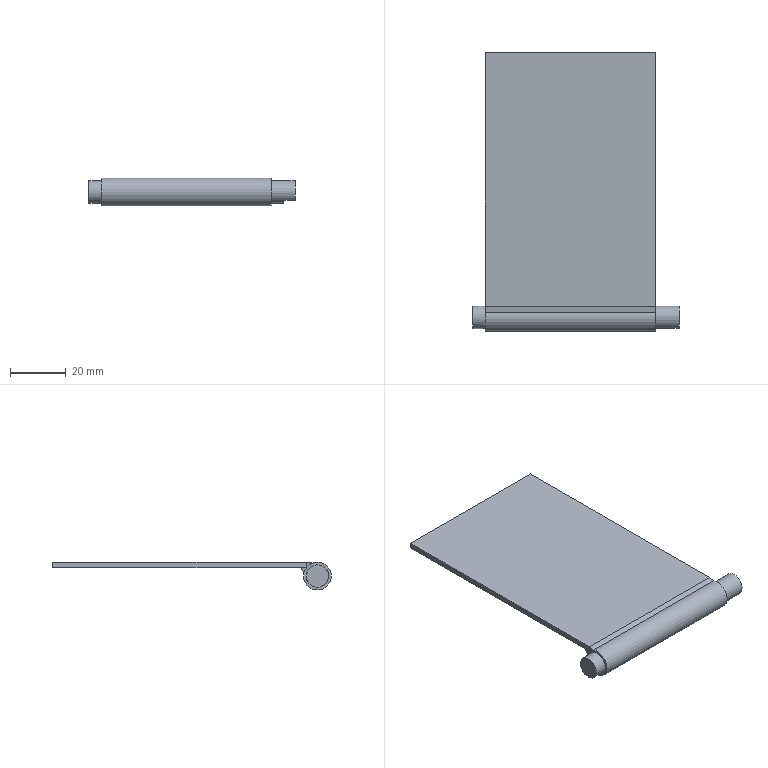Part | NX | features EXTRUDE 4, DATUM_CSYS 2, FSET 2, FILLET_WELD 1, HOLE PACKAGE 1, SIMPLE HOLE 1, SKETCH 1, SYMBOLIC_THREAD 1, WELD_GROOVE 1 | 4 solids | 28 faces | box 74 x 100 x 10 mm | volume 16601 mm3 | plane 19 | cylinder 6 | cone 2 | spline 1 | commonest cylinder face diameters 10 x3 8 x2 4.2 x1
STEP:
#1=CARTESIAN_POINT('',(-30.5,1.769,4.677));
#2=VERTEX_POINT('',#1);
#3=CARTESIAN_POINT('',(30.5,1.769,4.677));
#4=VERTEX_POINT('',#3);
#5=CARTESIAN_POINT('',(-0.000000001,1.769,4.677));
#6=DIRECTION('',(-1.,0.,0.));
#7=VECTOR('',#6,1000.);
#8=LINE('',#5,#7);
#9=EDGE_CURVE('',#2,#4,#8,.F.);
#10=ORIENTED_EDGE('',*,*,#9,.F.);
#11=CARTESIAN_POINT('',(-30.5,4.,3.));
#12=VERTEX_POINT('',#11);
#13=CARTESIAN_POINT('',(-30.5,0.,0.));
#14=DIRECTION('',(1.,0.,0.));
#15=DIRECTION('',(0.,1.,0.));
#16=AXIS2_PLACEMENT_3D('',#13,#14,#15);
#17=CIRCLE('',#16,5.);
#18=EDGE_CURVE('',#12,#2,#17,.T.);
#19=ORIENTED_EDGE('',*,*,#18,.F.);
#20=CARTESIAN_POINT('',(30.5,4.,3.));
#21=VERTEX_POINT('',#20);
#22=CARTESIAN_POINT('',(30.5,4.,3.));
#23=DIRECTION('',(-1.,0.,0.));
#24=VECTOR('',#23,1000.);
#25=LINE('',#22,#24);
#26=EDGE_CURVE('',#12,#21,#25,.F.);
#27=ORIENTED_EDGE('',*,*,#26,.T.);
#28=CARTESIAN_POINT('',(30.5,0.,0.));
#29=DIRECTION('',(1.,0.,0.));
#30=DIRECTION('',(0.,1.,0.));
#31=AXIS2_PLACEMENT_3D('',#28,#29,#30);
#32=CIRCLE('',#31,5.);
#33=EDGE_CURVE('',#21,#4,#32,.T.);
#34=ORIENTED_EDGE('',*,*,#33,.T.);
#35=EDGE_LOOP('',(#10,#19,#27,#34));
#36=FACE_BOUND('',#35,.T.);
#37=CARTESIAN_POINT('',(30.5,0.,0.));
#38=DIRECTION('',(-1.,0.,0.));
#39=DIRECTION('',(0.,0.,1.));
#40=AXIS2_PLACEMENT_3D('',#37,#38,#39);
#41=CYLINDRICAL_SURFACE('',#40,5.);
#42=ADVANCED_FACE('',(#36),#41,.F.);
#43=CARTESIAN_POINT('',(-30.5,4.,5.));
#44=VERTEX_POINT('',#43);
#45=CARTESIAN_POINT('',(-30.5,4.,3.));
#46=DIRECTION('',(0.,0.,1.));
#47=VECTOR('',#46,1000.);
#48=LINE('',#45,#47);
#49=EDGE_CURVE('',#12,#44,#48,.T.);
#50=ORIENTED_EDGE('',*,*,#49,.T.);
#51=CARTESIAN_POINT('',(30.5,4.,5.));
#52=VERTEX_POINT('',#51);
#53=CARTESIAN_POINT('',(-30.5,4.,5.));
#54=DIRECTION('',(1.,0.,0.));
#55=VECTOR('',#54,1000.);
#56=LINE('',#53,#55);
#57=EDGE_CURVE('',#44,#52,#56,.T.);
#58=ORIENTED_EDGE('',*,*,#57,.T.);
#59=CARTESIAN_POINT('',(30.5,4.,3.));
#60=DIRECTION('',(0.,0.,1.));
#61=VECTOR('',#60,1000.);
#62=LINE('',#59,#61);
#63=EDGE_CURVE('',#21,#52,#62,.T.);
#64=ORIENTED_EDGE('',*,*,#63,.F.);
#65=ORIENTED_EDGE('',*,*,#26,.F.);
#66=EDGE_LOOP('',(#50,#58,#64,#65));
#67=FACE_BOUND('',#66,.T.);
#68=CARTESIAN_POINT('',(-30.5,4.,3.));
#69=DIRECTION('',(0.,-1.,0.));
#70=DIRECTION('',(1.,0.,0.));
#71=AXIS2_PLACEMENT_3D('',#68,#69,#70);
#72=PLANE('',#71);
#73=ADVANCED_FACE('',(#67),#72,.F.);
#74=ORIENTED_EDGE('',*,*,#9,.T.);
#75=CARTESIAN_POINT('',(30.5,1.769,4.677));
#76=CARTESIAN_POINT('',(30.5,2.513,4.784));
#77=CARTESIAN_POINT('',(30.5,3.256,4.892));
#78=CARTESIAN_POINT('',(30.5,4.,5.));
#79=B_SPLINE_CURVE_WITH_KNOTS('',3,(#75,#76,#77,#78),.UNSPECIFIED.,.F.,.F.,(4,4),(0.,0.002254),.UNSPECIFIED.);
#80=EDGE_CURVE('',#4,#52,#79,.T.);
#81=ORIENTED_EDGE('',*,*,#80,.T.);
#82=ORIENTED_EDGE('',*,*,#57,.F.);
#83=CARTESIAN_POINT('',(-30.5,4.,5.));
#84=CARTESIAN_POINT('',(-30.5,3.256,4.892));
#85=CARTESIAN_POINT('',(-30.5,2.513,4.784));
#86=CARTESIAN_POINT('',(-30.5,1.769,4.677));
#87=B_SPLINE_CURVE_WITH_KNOTS('',3,(#83,#84,#85,#86),.UNSPECIFIED.,.F.,.F.,(4,4),(0.,0.002254),.UNSPECIFIED.);
#88=EDGE_CURVE('',#44,#2,#87,.T.);
#89=ORIENTED_EDGE('',*,*,#88,.T.);
#90=EDGE_LOOP('',(#74,#81,#82,#89));
#91=FACE_BOUND('',#90,.T.);
#92=CARTESIAN_POINT('',(-30.75,4.112,5.016));
#93=CARTESIAN_POINT('',(-30.75,3.293,4.898));
#94=CARTESIAN_POINT('',(-30.75,2.475,4.779));
#95=CARTESIAN_POINT('',(-30.75,1.657,4.66));
#96=CARTESIAN_POINT('',(-28.188,4.112,5.016));
#97=CARTESIAN_POINT('',(-28.187,3.293,4.898));
#98=CARTESIAN_POINT('',(-28.188,2.475,4.779));
#99=CARTESIAN_POINT('',(-28.187,1.657,4.66));
#100=CARTESIAN_POINT('',(-23.062,4.112,5.016));
#101=CARTESIAN_POINT('',(-23.063,3.293,4.898));
#102=CARTESIAN_POINT('',(-23.062,2.475,4.779));
#103=CARTESIAN_POINT('',(-23.062,1.657,4.66));
#104=CARTESIAN_POINT('',(-12.812,4.112,5.016));
#105=CARTESIAN_POINT('',(-12.813,3.293,4.898));
#106=CARTESIAN_POINT('',(-12.812,2.475,4.779));
#107=CARTESIAN_POINT('',(-12.813,1.657,4.66));
#108=CARTESIAN_POINT('',(-2.562,4.112,5.016));
#109=CARTESIAN_POINT('',(-2.563,3.293,4.898));
#110=CARTESIAN_POINT('',(-2.562,2.475,4.779));
#111=CARTESIAN_POINT('',(-2.563,1.657,4.66));
#112=CARTESIAN_POINT('',(7.687,4.112,5.016));
#113=CARTESIAN_POINT('',(7.688,3.293,4.898));
#114=CARTESIAN_POINT('',(7.687,2.475,4.779));
#115=CARTESIAN_POINT('',(7.687,1.657,4.66));
#116=CARTESIAN_POINT('',(15.375,4.112,5.016));
#117=CARTESIAN_POINT('',(15.375,3.293,4.898));
#118=CARTESIAN_POINT('',(15.375,2.475,4.779));
#119=CARTESIAN_POINT('',(15.375,1.657,4.66));
#120=CARTESIAN_POINT('',(23.062,4.112,5.016));
#121=CARTESIAN_POINT('',(23.063,3.293,4.898));
#122=CARTESIAN_POINT('',(23.062,2.475,4.779));
#123=CARTESIAN_POINT('',(23.062,1.657,4.66));
#124=CARTESIAN_POINT('',(28.188,4.112,5.016));
#125=CARTESIAN_POINT('',(28.187,3.293,4.898));
#126=CARTESIAN_POINT('',(28.188,2.475,4.779));
#127=CARTESIAN_POINT('',(28.187,1.657,4.66));
#128=CARTESIAN_POINT('',(30.75,4.112,5.016));
#129=CARTESIAN_POINT('',(30.75,3.293,4.898));
#130=CARTESIAN_POINT('',(30.75,2.475,4.779));
#131=CARTESIAN_POINT('',(30.75,1.657,4.66));
#132=B_SPLINE_SURFACE_WITH_KNOTS('',3,3,((#92,#93,#94,#95),(#96,#97,#98,#99),(#100,#101,#102,#103),(#104,#105,#106,#107),(#108,#109,#110,#111),(#112,#113,#114,#115),(#116,#117,#118,#119),(#120,#121,#122,#123),(#124,#125,#126,#127),(#128,#129,#130,#131)),.UNSPECIFIED.,.F.,.F.,.F.,(4,1,1,1,1,1,1,4),(4,4),(0.,0.125,0.25,0.5,0.625,0.75,0.875,1.),(0.,1.),.UNSPECIFIED.);
#133=ADVANCED_FACE('',(#91),#132,.F.);
#134=ORIENTED_EDGE('',*,*,#18,.T.);
#135=ORIENTED_EDGE('',*,*,#88,.F.);
#136=ORIENTED_EDGE('',*,*,#49,.F.);
#137=EDGE_LOOP('',(#134,#135,#136));
#138=FACE_BOUND('',#137,.T.);
#139=CARTESIAN_POINT('',(-30.5,4.,3.));
#140=DIRECTION('',(1.,0.,0.));
#141=DIRECTION('',(0.,0.,-1.));
#142=AXIS2_PLACEMENT_3D('',#139,#140,#141);
#143=PLANE('',#142);
#144=ADVANCED_FACE('',(#138),#143,.F.);
#145=ORIENTED_EDGE('',*,*,#33,.F.);
#146=ORIENTED_EDGE('',*,*,#63,.T.);
#147=ORIENTED_EDGE('',*,*,#80,.F.);
#148=EDGE_LOOP('',(#145,#146,#147));
#149=FACE_BOUND('',#148,.T.);
#150=CARTESIAN_POINT('',(30.5,4.,3.));
#151=DIRECTION('',(-1.,0.,0.));
#152=DIRECTION('',(0.,0.,1.));
#153=AXIS2_PLACEMENT_3D('',#150,#151,#152);
#154=PLANE('',#153);
#155=ADVANCED_FACE('',(#149),#154,.F.);
#156=CLOSED_SHELL('',(#42,#73,#133,#144,#155));
#157=MANIFOLD_SOLID_BREP('',#156);
#158=CARTESIAN_POINT('',(-30.5,95.,3.));
#159=VERTEX_POINT('',#158);
#160=CARTESIAN_POINT('',(-30.5,95.,5.));
#161=VERTEX_POINT('',#160);
#162=CARTESIAN_POINT('',(-30.5,95.,3.));
#163=DIRECTION('',(0.,0.,1.));
#164=VECTOR('',#163,1000.);
#165=LINE('',#162,#164);
#166=EDGE_CURVE('',#159,#161,#165,.T.);
#167=ORIENTED_EDGE('',*,*,#166,.F.);
#168=CARTESIAN_POINT('',(-30.5,4.,3.));
#169=VERTEX_POINT('',#168);
#170=CARTESIAN_POINT('',(-30.5,95.,3.));
#171=DIRECTION('',(0.,-1.,0.));
#172=VECTOR('',#171,1000.);
#173=LINE('',#170,#172);
#174=EDGE_CURVE('',#159,#169,#173,.T.);
#175=ORIENTED_EDGE('',*,*,#174,.T.);
#176=CARTESIAN_POINT('',(-30.5,4.,5.));
#177=VERTEX_POINT('',#176);
#178=CARTESIAN_POINT('',(-30.5,4.,3.));
#179=DIRECTION('',(0.,0.,1.));
#180=VECTOR('',#179,1000.);
#181=LINE('',#178,#180);
#182=EDGE_CURVE('',#169,#177,#181,.T.);
#183=ORIENTED_EDGE('',*,*,#182,.T.);
#184=CARTESIAN_POINT('',(-30.5,95.,5.));
#185=DIRECTION('',(0.,1.,0.));
#186=VECTOR('',#185,1000.);
#187=LINE('',#184,#186);
#188=EDGE_CURVE('',#161,#177,#187,.F.);
#189=ORIENTED_EDGE('',*,*,#188,.F.);
#190=EDGE_LOOP('',(#167,#175,#183,#189));
#191=FACE_BOUND('',#190,.T.);
#192=CARTESIAN_POINT('',(-30.5,95.,3.));
#193=DIRECTION('',(-1.,0.,0.));
#194=DIRECTION('',(0.,-1.,0.));
#195=AXIS2_PLACEMENT_3D('',#192,#193,#194);
#196=PLANE('',#195);
#197=ADVANCED_FACE('',(#191),#196,.T.);
#198=ORIENTED_EDGE('',*,*,#182,.F.);
#199=CARTESIAN_POINT('',(30.5,4.,3.));
#200=VERTEX_POINT('',#199);
#201=CARTESIAN_POINT('',(-30.5,4.,3.));
#202=DIRECTION('',(1.,0.,0.));
#203=VECTOR('',#202,1000.);
#204=LINE('',#201,#203);
#205=EDGE_CURVE('',#169,#200,#204,.T.);
#206=ORIENTED_EDGE('',*,*,#205,.T.);
#207=CARTESIAN_POINT('',(30.5,4.,5.));
#208=VERTEX_POINT('',#207);
#209=CARTESIAN_POINT('',(30.5,4.,3.));
#210=DIRECTION('',(0.,0.,1.));
#211=VECTOR('',#210,1000.);
#212=LINE('',#209,#211);
#213=EDGE_CURVE('',#200,#208,#212,.T.);
#214=ORIENTED_EDGE('',*,*,#213,.T.);
#215=CARTESIAN_POINT('',(-30.5,4.,5.));
#216=DIRECTION('',(1.,0.,0.));
#217=VECTOR('',#216,1000.);
#218=LINE('',#215,#217);
#219=EDGE_CURVE('',#177,#208,#218,.T.);
#220=ORIENTED_EDGE('',*,*,#219,.F.);
#221=EDGE_LOOP('',(#198,#206,#214,#220));
#222=FACE_BOUND('',#221,.T.);
#223=CARTESIAN_POINT('',(-30.5,4.,3.));
#224=DIRECTION('',(0.,-1.,0.));
#225=DIRECTION('',(1.,0.,0.));
#226=AXIS2_PLACEMENT_3D('',#223,#224,#225);
#227=PLANE('',#226);
#228=ADVANCED_FACE('',(#222),#227,.T.);
#229=ORIENTED_EDGE('',*,*,#213,.F.);
#230=CARTESIAN_POINT('',(30.5,95.,3.));
#231=VERTEX_POINT('',#230);
#232=CARTESIAN_POINT('',(30.5,95.,3.));
#233=DIRECTION('',(0.,-1.,0.));
#234=VECTOR('',#233,1000.);
#235=LINE('',#232,#234);
#236=EDGE_CURVE('',#231,#200,#235,.T.);
#237=ORIENTED_EDGE('',*,*,#236,.F.);
#238=CARTESIAN_POINT('',(30.5,95.,5.));
#239=VERTEX_POINT('',#238);
#240=CARTESIAN_POINT('',(30.5,95.,3.));
#241=DIRECTION('',(0.,0.,1.));
#242=VECTOR('',#241,1000.);
#243=LINE('',#240,#242);
#244=EDGE_CURVE('',#231,#239,#243,.T.);
#245=ORIENTED_EDGE('',*,*,#244,.T.);
#246=CARTESIAN_POINT('',(30.5,95.,5.));
#247=DIRECTION('',(0.,1.,0.));
#248=VECTOR('',#247,1000.);
#249=LINE('',#246,#248);
#250=EDGE_CURVE('',#239,#208,#249,.F.);
#251=ORIENTED_EDGE('',*,*,#250,.T.);
#252=EDGE_LOOP('',(#229,#237,#245,#251));
#253=FACE_BOUND('',#252,.T.);
#254=CARTESIAN_POINT('',(30.5,95.,3.));
#255=DIRECTION('',(-1.,0.,0.));
#256=DIRECTION('',(0.,-1.,0.));
#257=AXIS2_PLACEMENT_3D('',#254,#255,#256);
#258=PLANE('',#257);
#259=ADVANCED_FACE('',(#253),#258,.F.);
#260=CARTESIAN_POINT('',(-30.5,95.,3.));
#261=DIRECTION('',(1.,0.,0.));
#262=VECTOR('',#261,1000.);
#263=LINE('',#260,#262);
#264=EDGE_CURVE('',#159,#231,#263,.T.);
#265=ORIENTED_EDGE('',*,*,#264,.F.);
#266=ORIENTED_EDGE('',*,*,#166,.T.);
#267=CARTESIAN_POINT('',(-30.5,95.,5.));
#268=DIRECTION('',(1.,0.,0.));
#269=VECTOR('',#268,1000.);
#270=LINE('',#267,#269);
#271=EDGE_CURVE('',#161,#239,#270,.T.);
#272=ORIENTED_EDGE('',*,*,#271,.T.);
#273=ORIENTED_EDGE('',*,*,#244,.F.);
#274=EDGE_LOOP('',(#265,#266,#272,#273));
#275=FACE_BOUND('',#274,.T.);
#276=CARTESIAN_POINT('',(-30.5,95.,3.));
#277=DIRECTION('',(0.,-1.,0.));
#278=DIRECTION('',(1.,0.,0.));
#279=AXIS2_PLACEMENT_3D('',#276,#277,#278);
#280=PLANE('',#279);
#281=ADVANCED_FACE('',(#275),#280,.F.);
#282=ORIENTED_EDGE('',*,*,#250,.F.);
#283=ORIENTED_EDGE('',*,*,#271,.F.);
#284=ORIENTED_EDGE('',*,*,#188,.T.);
#285=ORIENTED_EDGE('',*,*,#219,.T.);
#286=EDGE_LOOP('',(#282,#283,#284,#285));
#287=FACE_BOUND('',#286,.T.);
#288=CARTESIAN_POINT('',(-30.5,95.,5.));
#289=DIRECTION('',(0.,0.,1.));
#290=DIRECTION('',(1.,0.,0.));
#291=AXIS2_PLACEMENT_3D('',#288,#289,#290);
#292=PLANE('',#291);
#293=ADVANCED_FACE('',(#287),#292,.T.);
#294=ORIENTED_EDGE('',*,*,#236,.T.);
#295=ORIENTED_EDGE('',*,*,#205,.F.);
#296=ORIENTED_EDGE('',*,*,#174,.F.);
#297=ORIENTED_EDGE('',*,*,#264,.T.);
#298=EDGE_LOOP('',(#294,#295,#296,#297));
#299=FACE_BOUND('',#298,.T.);
#300=CARTESIAN_POINT('',(-30.5,95.,3.));
#301=DIRECTION('',(0.,0.,1.));
#302=DIRECTION('',(1.,0.,0.));
#303=AXIS2_PLACEMENT_3D('',#300,#301,#302);
#304=PLANE('',#303);
#305=ADVANCED_FACE('',(#299),#304,.F.);
#306=CLOSED_SHELL('',(#197,#228,#259,#281,#293,#305));
#307=MANIFOLD_SOLID_BREP('',#306);
#308=CARTESIAN_POINT('',(-30.5,6.,3.));
#309=VERTEX_POINT('',#308);
#310=CARTESIAN_POINT('',(-30.5,4.,3.));
#311=VERTEX_POINT('',#310);
#312=CARTESIAN_POINT('',(-30.5,95.,3.));
#313=DIRECTION('',(0.,-1.,0.));
#314=VECTOR('',#313,1000.);
#315=LINE('',#312,#314);
#316=EDGE_CURVE('',#309,#311,#315,.T.);
#317=ORIENTED_EDGE('',*,*,#316,.F.);
#318=CARTESIAN_POINT('',(-30.5,4.852,1.206));
#319=VERTEX_POINT('',#318);
#320=CARTESIAN_POINT('',(-30.5,5.426,2.103));
#321=DIRECTION('',(0.,-0.5387,-0.8425));
#322=VECTOR('',#321,1000.);
#323=LINE('',#320,#322);
#324=EDGE_CURVE('',#309,#319,#323,.T.);
#325=ORIENTED_EDGE('',*,*,#324,.T.);
#326=CARTESIAN_POINT('',(-30.5,0.,0.));
#327=DIRECTION('',(1.,0.,0.));
#328=DIRECTION('',(0.,1.,0.));
#329=AXIS2_PLACEMENT_3D('',#326,#327,#328);
#330=CIRCLE('',#329,5.);
#331=EDGE_CURVE('',#319,#311,#330,.T.);
#332=ORIENTED_EDGE('',*,*,#331,.T.);
#333=EDGE_LOOP('',(#317,#325,#332));
#334=FACE_BOUND('',#333,.T.);
#335=CARTESIAN_POINT('',(-30.5,4.,3.));
#336=DIRECTION('',(1.,0.,0.));
#337=DIRECTION('',(0.,1.,0.));
#338=AXIS2_PLACEMENT_3D('',#335,#336,#337);
#339=PLANE('',#338);
#340=ADVANCED_FACE('',(#334),#339,.F.);
#341=CARTESIAN_POINT('',(30.5,6.,3.));
#342=VERTEX_POINT('',#341);
#343=CARTESIAN_POINT('',(30.5,4.,3.));
#344=VERTEX_POINT('',#343);
#345=CARTESIAN_POINT('',(30.5,95.,3.));
#346=DIRECTION('',(0.,-1.,0.));
#347=VECTOR('',#346,1000.);
#348=LINE('',#345,#347);
#349=EDGE_CURVE('',#342,#344,#348,.T.);
#350=ORIENTED_EDGE('',*,*,#349,.T.);
#351=CARTESIAN_POINT('',(30.5,4.852,1.206));
#352=VERTEX_POINT('',#351);
#353=CARTESIAN_POINT('',(30.5,0.,0.));
#354=DIRECTION('',(1.,0.,0.));
#355=DIRECTION('',(0.,1.,0.));
#356=AXIS2_PLACEMENT_3D('',#353,#354,#355);
#357=CIRCLE('',#356,5.);
#358=EDGE_CURVE('',#352,#344,#357,.T.);
#359=ORIENTED_EDGE('',*,*,#358,.F.);
#360=CARTESIAN_POINT('',(30.5,5.426,2.103));
#361=DIRECTION('',(0.,0.5387,0.8425));
#362=VECTOR('',#361,1000.);
#363=LINE('',#360,#362);
#364=EDGE_CURVE('',#352,#342,#363,.T.);
#365=ORIENTED_EDGE('',*,*,#364,.T.);
#366=EDGE_LOOP('',(#350,#359,#365));
#367=FACE_BOUND('',#366,.T.);
#368=CARTESIAN_POINT('',(30.5,4.,3.));
#369=DIRECTION('',(-1.,0.,0.));
#370=DIRECTION('',(0.,0.,1.));
#371=AXIS2_PLACEMENT_3D('',#368,#369,#370);
#372=PLANE('',#371);
#373=ADVANCED_FACE('',(#367),#372,.F.);
#374=ORIENTED_EDGE('',*,*,#324,.F.);
#375=CARTESIAN_POINT('',(0.,6.,3.));
#376=DIRECTION('',(-1.,0.,0.));
#377=VECTOR('',#376,1000.);
#378=LINE('',#375,#377);
#379=EDGE_CURVE('',#309,#342,#378,.F.);
#380=ORIENTED_EDGE('',*,*,#379,.T.);
#381=ORIENTED_EDGE('',*,*,#364,.F.);
#382=CARTESIAN_POINT('',(0.,4.852,1.206));
#383=DIRECTION('',(-1.,0.,0.));
#384=VECTOR('',#383,1000.);
#385=LINE('',#382,#384);
#386=EDGE_CURVE('',#352,#319,#385,.T.);
#387=ORIENTED_EDGE('',*,*,#386,.T.);
#388=EDGE_LOOP('',(#374,#380,#381,#387));
#389=FACE_BOUND('',#388,.T.);
#390=CARTESIAN_POINT('',(30.5,6.076,3.119));
#391=DIRECTION('',(0.,-0.8425,0.5387));
#392=DIRECTION('',(-1.,0.,0.));
#393=AXIS2_PLACEMENT_3D('',#390,#391,#392);
#394=PLANE('',#393);
#395=ADVANCED_FACE('',(#389),#394,.F.);
#396=ORIENTED_EDGE('',*,*,#358,.T.);
#397=CARTESIAN_POINT('',(-30.5,4.,3.));
#398=DIRECTION('',(1.,0.,0.));
#399=VECTOR('',#398,1000.);
#400=LINE('',#397,#399);
#401=EDGE_CURVE('',#311,#344,#400,.T.);
#402=ORIENTED_EDGE('',*,*,#401,.F.);
#403=ORIENTED_EDGE('',*,*,#331,.F.);
#404=ORIENTED_EDGE('',*,*,#386,.F.);
#405=EDGE_LOOP('',(#396,#402,#403,#404));
#406=FACE_BOUND('',#405,.T.);
#407=CARTESIAN_POINT('',(30.5,0.,0.));
#408=DIRECTION('',(-1.,0.,0.));
#409=DIRECTION('',(0.,0.,1.));
#410=AXIS2_PLACEMENT_3D('',#407,#408,#409);
#411=CYLINDRICAL_SURFACE('',#410,5.);
#412=ADVANCED_FACE('',(#406),#411,.F.);
#413=ORIENTED_EDGE('',*,*,#316,.T.);
#414=ORIENTED_EDGE('',*,*,#401,.T.);
#415=ORIENTED_EDGE('',*,*,#349,.F.);
#416=ORIENTED_EDGE('',*,*,#379,.F.);
#417=EDGE_LOOP('',(#413,#414,#415,#416));
#418=FACE_BOUND('',#417,.T.);
#419=CARTESIAN_POINT('',(-30.5,95.,3.));
#420=DIRECTION('',(0.,0.,1.));
#421=DIRECTION('',(1.,0.,0.));
#422=AXIS2_PLACEMENT_3D('',#419,#420,#421);
#423=PLANE('',#422);
#424=ADVANCED_FACE('',(#418),#423,.T.);
#425=CLOSED_SHELL('',(#340,#373,#395,#412,#424));
#426=MANIFOLD_SOLID_BREP('',#425);
#427=CARTESIAN_POINT('',(35.,-2.646,-3.));
#428=VERTEX_POINT('',#427);
#429=CARTESIAN_POINT('',(35.,2.646,-3.));
#430=VERTEX_POINT('',#429);
#431=CARTESIAN_POINT('',(35.,2.646,-3.));
#432=DIRECTION('',(0.,1.,0.));
#433=VECTOR('',#432,1000.);
#434=LINE('',#431,#433);
#435=EDGE_CURVE('',#428,#430,#434,.T.);
#436=ORIENTED_EDGE('',*,*,#435,.F.);
#437=CARTESIAN_POINT('',(35.,0.,0.));
#438=DIRECTION('',(-1.,0.,0.));
#439=DIRECTION('',(0.,1.,0.));
#440=AXIS2_PLACEMENT_3D('',#437,#438,#439);
#441=CIRCLE('',#440,4.);
#442=EDGE_CURVE('',#430,#428,#441,.T.);
#443=ORIENTED_EDGE('',*,*,#442,.F.);
#444=EDGE_LOOP('',(#436,#443));
#445=FACE_BOUND('',#444,.T.);
#446=CARTESIAN_POINT('',(35.,0.,0.));
#447=DIRECTION('',(-1.,0.,0.));
#448=DIRECTION('',(0.,0.,1.));
#449=AXIS2_PLACEMENT_3D('',#446,#447,#448);
#450=PLANE('',#449);
#451=ADVANCED_FACE('',(#445),#450,.F.);
#452=CARTESIAN_POINT('',(30.5,5.,0.));
#453=VERTEX_POINT('',#452);
#454=CARTESIAN_POINT('',(30.5,0.,0.));
#455=DIRECTION('',(1.,0.,0.));
#456=DIRECTION('',(0.,1.,0.));
#457=AXIS2_PLACEMENT_3D('',#454,#455,#456);
#458=CIRCLE('',#457,5.);
#459=EDGE_CURVE('',#453,#453,#458,.T.);
#460=ORIENTED_EDGE('',*,*,#459,.F.);
#461=EDGE_LOOP('',(#460));
#462=FACE_BOUND('',#461,.T.);
#463=CARTESIAN_POINT('',(-30.5,5.,0.));
#464=VERTEX_POINT('',#463);
#465=CARTESIAN_POINT('',(-30.5,0.,0.));
#466=DIRECTION('',(1.,0.,0.));
#467=DIRECTION('',(0.,1.,0.));
#468=AXIS2_PLACEMENT_3D('',#465,#466,#467);
#469=CIRCLE('',#468,5.);
#470=EDGE_CURVE('',#464,#464,#469,.T.);
#471=ORIENTED_EDGE('',*,*,#470,.T.);
#472=EDGE_LOOP('',(#471));
#473=FACE_BOUND('',#472,.T.);
#474=CARTESIAN_POINT('',(30.5,0.,0.));
#475=DIRECTION('',(-1.,0.,0.));
#476=DIRECTION('',(0.,0.,1.));
#477=AXIS2_PLACEMENT_3D('',#474,#475,#476);
#478=CYLINDRICAL_SURFACE('',#477,5.);
#479=ADVANCED_FACE('',(#462,#473),#478,.T.);
#480=CARTESIAN_POINT('',(30.5,0.,-4.));
#481=VERTEX_POINT('',#480);
#482=CARTESIAN_POINT('',(30.5,0.,0.));
#483=DIRECTION('',(1.,0.,0.));
#484=DIRECTION('',(0.,0.,-1.));
#485=AXIS2_PLACEMENT_3D('',#482,#483,#484);
#486=CIRCLE('',#485,4.);
#487=EDGE_CURVE('',#481,#481,#486,.F.);
#488=ORIENTED_EDGE('',*,*,#487,.T.);
#489=EDGE_LOOP('',(#488));
#490=FACE_BOUND('',#489,.T.);
#491=ORIENTED_EDGE('',*,*,#459,.T.);
#492=EDGE_LOOP('',(#491));
#493=FACE_BOUND('',#492,.T.);
#494=CARTESIAN_POINT('',(30.5,0.,0.));
#495=DIRECTION('',(1.,0.,0.));
#496=DIRECTION('',(0.,0.,-1.));
#497=AXIS2_PLACEMENT_3D('',#494,#495,#496);
#498=PLANE('',#497);
#499=ADVANCED_FACE('',(#490,#493),#498,.T.);
#500=CARTESIAN_POINT('',(-30.5,0.,-4.));
#501=VERTEX_POINT('',#500);
#502=CARTESIAN_POINT('',(-30.5,0.,0.));
#503=DIRECTION('',(1.,0.,0.));
#504=DIRECTION('',(0.,0.,-1.));
#505=AXIS2_PLACEMENT_3D('',#502,#503,#504);
#506=CIRCLE('',#505,4.);
#507=EDGE_CURVE('',#501,#501,#506,.F.);
#508=ORIENTED_EDGE('',*,*,#507,.F.);
#509=EDGE_LOOP('',(#508));
#510=FACE_BOUND('',#509,.T.);
#511=ORIENTED_EDGE('',*,*,#470,.F.);
#512=EDGE_LOOP('',(#511));
#513=FACE_BOUND('',#512,.T.);
#514=CARTESIAN_POINT('',(-30.5,0.,0.));
#515=DIRECTION('',(1.,0.,0.));
#516=DIRECTION('',(0.,0.,-1.));
#517=AXIS2_PLACEMENT_3D('',#514,#515,#516);
#518=PLANE('',#517);
#519=ADVANCED_FACE('',(#510,#513),#518,.F.);
#520=CARTESIAN_POINT('',(-35.,4.,0.));
#521=VERTEX_POINT('',#520);
#522=CARTESIAN_POINT('',(-35.,0.,0.));
#523=DIRECTION('',(-1.,0.,0.));
#524=DIRECTION('',(0.,1.,0.));
#525=AXIS2_PLACEMENT_3D('',#522,#523,#524);
#526=CIRCLE('',#525,4.);
#527=EDGE_CURVE('',#521,#521,#526,.T.);
#528=ORIENTED_EDGE('',*,*,#527,.T.);
#529=EDGE_LOOP('',(#528));
#530=FACE_BOUND('',#529,.T.);
#531=CARTESIAN_POINT('',(-35.,0.,0.));
#532=DIRECTION('',(-1.,0.,0.));
#533=DIRECTION('',(0.,0.,1.));
#534=AXIS2_PLACEMENT_3D('',#531,#532,#533);
#535=PLANE('',#534);
#536=ADVANCED_FACE('',(#530),#535,.T.);
#537=ORIENTED_EDGE('',*,*,#527,.F.);
#538=EDGE_LOOP('',(#537));
#539=FACE_BOUND('',#538,.T.);
#540=ORIENTED_EDGE('',*,*,#507,.T.);
#541=EDGE_LOOP('',(#540));
#542=FACE_BOUND('',#541,.T.);
#543=CARTESIAN_POINT('',(-35.,0.,0.));
#544=DIRECTION('',(1.,0.,0.));
#545=DIRECTION('',(0.,0.,-1.));
#546=AXIS2_PLACEMENT_3D('',#543,#544,#545);
#547=CYLINDRICAL_SURFACE('',#546,4.);
#548=ADVANCED_FACE('',(#539,#542),#547,.T.);
#549=ORIENTED_EDGE('',*,*,#487,.F.);
#550=EDGE_LOOP('',(#549));
#551=FACE_BOUND('',#550,.T.);
#552=ORIENTED_EDGE('',*,*,#442,.T.);
#553=CARTESIAN_POINT('',(39.,-2.646,-3.));
#554=VERTEX_POINT('',#553);
#555=CARTESIAN_POINT('',(351.,-2.646,-3.));
#556=DIRECTION('',(-1.,0.,0.));
#557=VECTOR('',#556,1000.);
#558=LINE('',#555,#557);
#559=EDGE_CURVE('',#428,#554,#558,.F.);
#560=ORIENTED_EDGE('',*,*,#559,.T.);
#561=CARTESIAN_POINT('',(39.,2.646,-3.));
#562=VERTEX_POINT('',#561);
#563=CARTESIAN_POINT('',(39.,0.,0.));
#564=DIRECTION('',(-1.,0.,0.));
#565=DIRECTION('',(0.,0.,1.));
#566=AXIS2_PLACEMENT_3D('',#563,#564,#565);
#567=CIRCLE('',#566,4.);
#568=EDGE_CURVE('',#562,#554,#567,.F.);
#569=ORIENTED_EDGE('',*,*,#568,.F.);
#570=CARTESIAN_POINT('',(351.,2.646,-3.));
#571=DIRECTION('',(-1.,0.,0.));
#572=VECTOR('',#571,1000.);
#573=LINE('',#570,#572);
#574=EDGE_CURVE('',#562,#430,#573,.T.);
#575=ORIENTED_EDGE('',*,*,#574,.T.);
#576=EDGE_LOOP('',(#552,#560,#569,#575));
#577=FACE_BOUND('',#576,.T.);
#578=CARTESIAN_POINT('',(-35.,0.,0.));
#579=DIRECTION('',(1.,0.,0.));
#580=DIRECTION('',(0.,0.,-1.));
#581=AXIS2_PLACEMENT_3D('',#578,#579,#580);
#582=CYLINDRICAL_SURFACE('',#581,4.);
#583=ADVANCED_FACE('',(#551,#577),#582,.T.);
#584=CARTESIAN_POINT('',(39.,2.646,-3.));
#585=DIRECTION('',(0.,1.,0.));
#586=VECTOR('',#585,1000.);
#587=LINE('',#584,#586);
#588=EDGE_CURVE('',#554,#562,#587,.T.);
#589=ORIENTED_EDGE('',*,*,#588,.F.);
#590=ORIENTED_EDGE('',*,*,#559,.F.);
#591=ORIENTED_EDGE('',*,*,#435,.T.);
#592=ORIENTED_EDGE('',*,*,#574,.F.);
#593=EDGE_LOOP('',(#589,#590,#591,#592));
#594=FACE_BOUND('',#593,.T.);
#595=CARTESIAN_POINT('',(351.,2.646,-3.));
#596=DIRECTION('',(0.,0.,-1.));
#597=DIRECTION('',(-1.,0.,0.));
#598=AXIS2_PLACEMENT_3D('',#595,#596,#597);
#599=PLANE('',#598);
#600=ADVANCED_FACE('',(#594),#599,.T.);
#601=CARTESIAN_POINT('',(39.,0.,2.5));
#602=VERTEX_POINT('',#601);
#603=CARTESIAN_POINT('',(39.,0.,0.));
#604=DIRECTION('',(-1.,0.,0.));
#605=DIRECTION('',(0.,0.,1.));
#606=AXIS2_PLACEMENT_3D('',#603,#604,#605);
#607=CIRCLE('',#606,2.5);
#608=EDGE_CURVE('',#602,#602,#607,.T.);
#609=ORIENTED_EDGE('',*,*,#608,.T.);
#610=EDGE_LOOP('',(#609));
#611=FACE_BOUND('',#610,.T.);
#612=ORIENTED_EDGE('',*,*,#588,.T.);
#613=ORIENTED_EDGE('',*,*,#568,.T.);
#614=EDGE_LOOP('',(#612,#613));
#615=FACE_BOUND('',#614,.T.);
#616=CARTESIAN_POINT('',(39.,0.,0.));
#617=DIRECTION('',(-1.,0.,0.));
#618=DIRECTION('',(0.,0.,1.));
#619=AXIS2_PLACEMENT_3D('',#616,#617,#618);
#620=PLANE('',#619);
#621=ADVANCED_FACE('',(#611,#615),#620,.F.);
#622=ORIENTED_EDGE('',*,*,#608,.F.);
#623=EDGE_LOOP('',(#622));
#624=FACE_BOUND('',#623,.T.);
#625=CARTESIAN_POINT('',(38.6,0.,-2.1));
#626=VERTEX_POINT('',#625);
#627=CARTESIAN_POINT('',(38.6,0.,0.));
#628=DIRECTION('',(1.,0.,0.));
#629=DIRECTION('',(0.,0.,-1.));
#630=AXIS2_PLACEMENT_3D('',#627,#628,#629);
#631=CIRCLE('',#630,2.1);
#632=EDGE_CURVE('',#626,#626,#631,.T.);
#633=ORIENTED_EDGE('',*,*,#632,.F.);
#634=EDGE_LOOP('',(#633));
#635=FACE_BOUND('',#634,.T.);
#636=CARTESIAN_POINT('',(36.5,0.,0.));
#637=DIRECTION('',(1.,0.,0.));
#638=DIRECTION('',(0.,1.,0.));
#639=AXIS2_PLACEMENT_3D('',#636,#637,#638);
#640=CONICAL_SURFACE('',#639,0.,0.7854);
#641=ADVANCED_FACE('',(#624,#635),#640,.F.);
#642=CARTESIAN_POINT('',(29.,0.,2.1));
#643=VERTEX_POINT('',#642);
#644=CARTESIAN_POINT('',(29.,0.,0.));
#645=DIRECTION('',(-1.,0.,0.));
#646=DIRECTION('',(0.,0.,1.));
#647=AXIS2_PLACEMENT_3D('',#644,#645,#646);
#648=CIRCLE('',#647,2.1);
#649=EDGE_CURVE('',#643,#643,#648,.F.);
#650=ORIENTED_EDGE('',*,*,#649,.T.);
#651=EDGE_LOOP('',(#650));
#652=FACE_BOUND('',#651,.T.);
#653=CARTESIAN_POINT('',(27.738,0.,0.));
#654=VERTEX_POINT('',#653);
#655=VERTEX_LOOP('',#654);
#656=FACE_BOUND('',#655,.T.);
#657=CARTESIAN_POINT('',(29.,0.,0.));
#658=DIRECTION('',(1.,0.,0.));
#659=DIRECTION('',(0.,0.,-1.));
#660=AXIS2_PLACEMENT_3D('',#657,#658,#659);
#661=CONICAL_SURFACE('',#660,2.1,1.03);
#662=ADVANCED_FACE('',(#652,#656),#661,.F.);
#663=ORIENTED_EDGE('',*,*,#632,.T.);
#664=EDGE_LOOP('',(#663));
#665=FACE_BOUND('',#664,.T.);
#666=ORIENTED_EDGE('',*,*,#649,.F.);
#667=EDGE_LOOP('',(#666));
#668=FACE_BOUND('',#667,.T.);
#669=CARTESIAN_POINT('',(39.,0.,0.));
#670=DIRECTION('',(-1.,0.,0.));
#671=DIRECTION('',(0.,0.,1.));
#672=AXIS2_PLACEMENT_3D('',#669,#670,#671);
#673=CYLINDRICAL_SURFACE('',#672,2.1);
#674=ADVANCED_FACE('',(#665,#668),#673,.F.);
#675=CLOSED_SHELL('',(#451,#479,#499,#519,#536,#548,#583,#600,#621,#641,#662,#674));
#676=MANIFOLD_SOLID_BREP('',#675);
#677=(LENGTH_UNIT()NAMED_UNIT(*)SI_UNIT(.MILLI.,.METRE.));
#678=UNCERTAINTY_MEASURE_WITH_UNIT(LENGTH_MEASURE(0.0508),#677,'','');
#679=(NAMED_UNIT(*)PLANE_ANGLE_UNIT()SI_UNIT($,.RADIAN.));
#680=(NAMED_UNIT(*)SI_UNIT($,.STERADIAN.)SOLID_ANGLE_UNIT());
#681=(GEOMETRIC_REPRESENTATION_CONTEXT(3)GLOBAL_UNCERTAINTY_ASSIGNED_CONTEXT((#678))GLOBAL_UNIT_ASSIGNED_CONTEXT((#677,#679,#680))REPRESENTATION_CONTEXT('',''));
#682=ADVANCED_BREP_SHAPE_REPRESENTATION('',(#157,#307,#426,#676),#681);